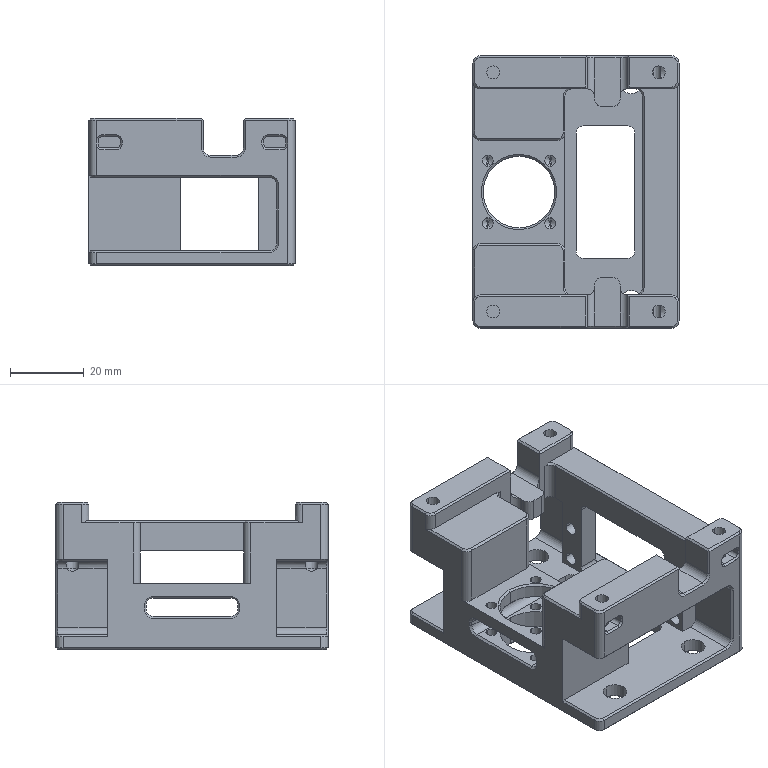NC program | Mastercam | posted with a generic post | part box 56 x 74 x 40 mm
Lines 2694 to 4682 of 45205, first 1710 of 1989 lines:
(4 FEM |TOOL - 4|DIA. OFF. - 4|LEN. - 4|TOOL DIA. - 4.)
N5436 T4 M6
N5438 G0 G54 G90 X22.359 Y9.943 C0. B0. S7000 M3
N5440 G43 H4 Z50.
N5442 Z3.054
N5444 G1 Z2.554 F600.
N5446 X22.37 Z2.345 F3000.
N5448 X22.402 Z2.138
N5450 X22.456 Z1.936
N5452 X22.531 Z1.74
N5454 X22.627 Z1.554
N5456 X22.741 Z1.378
N5458 X22.872 Z1.216
N5460 X23.02 Z1.068
N5462 X23.183 Z.936
N5464 X23.359 Z.822
N5466 X23.545 Z.727
N5468 X23.741 Z.652
N5470 X23.943 Z.598
N5472 X24.15 Z.565
N5474 X24.359 Z.554
N5476 X24.568 Y9.954 Z.517
N5478 X24.774 Y9.987 Z.48
N5480 X24.977 Y10.041 Z.443
N5482 X25.172 Y10.116 Z.406
N5484 X25.359 Y10.211 Z.369
N5486 X25.534 Y10.325 Z.332
N5488 X25.697 Y10.457 Z.295
N5490 X25.845 Y10.605 Z.259
N5492 X25.977 Y10.768 Z.222
N5494 X26.091 Y10.943 Z.185
N5496 X26.186 Y11.13 Z.148
N5498 X26.261 Y11.325 Z.111
N5500 X26.315 Y11.527 Z.074
N5502 X26.348 Y11.734 Z.037
N5504 X26.359 Y11.943 Z0.
N5506 Y13.91
N5508 X26.345 Y14.061
N5510 X26.304 Y14.175
N5512 X26.225 Y14.269
N5514 X26.061 Y14.345
N5516 X24.136 Y14.359
N5518 X24.077 Y14.358 Z-.001
N5520 X24.017 Y14.355 Z-.004
N5522 X23.958 Y14.35 Z-.01
N5524 X23.9 Y14.343 Z-.017
N5526 X23.843 Y14.335 Z-.026
N5528 X23.787 Y14.324 Z-.036
N5530 X23.732 Y14.313 Z-.048
N5532 X23.678 Y14.3 Z-.061
N5534 X23.627 Y14.286 Z-.075
N5536 X23.578 Y14.27 Z-.09
N5538 X23.531 Y14.254 Z-.106
N5540 X23.486 Y14.237 Z-.123
N5542 X23.444 Y14.22 Z-.14
N5544 X23.406 Y14.202 Z-.158
N5546 X23.37 Y14.184 Z-.176
N5548 X23.338 Y14.166 Z-.194
N5550 X23.31 Y14.147 Z-.213
N5552 X23.286 Y14.129 Z-.231
N5554 X23.265 Y14.111 Z-.248
N5556 X23.25 Y14.094 Z-.266
N5558 X23.239 Y14.077 Z-.283
N5560 X23.235 Y14.069 Z-.291
N5562 X23.233 Y14.061 Z-.299
N5564 X23.231 Y14.053 Z-.306
N5566 X23.232 Y14.045 Z-.314
N5568 X23.233 Y14.038 Z-.321
N5570 X23.236 Y14.031 Z-.328
N5572 X23.24 Y14.024 Z-.335
N5574 X23.246 Y14.018 Z-.341
N5576 X23.253 Y14.012 Z-.347
N5578 X23.262 Y14.006 Z-.353
N5580 X23.272 Y14.001 Z-.358
N5582 X23.284 Y13.995 Z-.363
N5584 X23.312 Y13.987 Z-.372
N5586 X23.347 Y13.979 Z-.379
N5588 X23.388 Y13.974 Z-.385
N5590 X23.437 Y13.971 Z-.388
N5592 X23.493 Y13.97 Z-.389
N5594 X25.91
N5596 X25.965 Y13.965
N5598 X25.97 Y13.908
N5600 Y11.623
N5602 X25.969 Y11.571 Z-.393
N5604 X25.967 Y11.569 Z-.394
N5606 Y11.568
N5608 Y11.565
N5610 Y11.559 Z-.395
N5612 X25.965 Y11.547 Z-.398
N5614 X25.96 Y11.526 Z-.402
N5616 X25.95 Y11.488 Z-.412
N5618 X25.934 Y11.456 Z-.428
N5620 X25.927 Y11.432 Z-.435
N5622 X25.921 Y11.415 Z-.443
N5624 X25.915 Y11.404 Z-.452
N5626 X25.912 Y11.402 Z-.459
N5628 X25.909 Y11.401 Z-.466
N5630 X25.905 Y11.402 Z-.477
N5632 X25.903 Y11.404 Z-.62
N5634 Y11.415 Z-.655
N5636 X25.902 Y11.432 Z-.688
N5638 Y11.456 Z-.717
N5640 Y11.488 Z-.742
N5642 X25.901 Y11.526 Z-.761
N5644 Y11.531 Z-.763
N5646 X25.903 Y11.532
N5648 X25.902 Y11.534 Z-.764
N5650 Y11.536 Z-.765
N5652 Y11.547 Z-.768
N5654 X25.901 Y11.571 Z-.773
N5656 X25.9 Y11.623 Z-.778
N5658 Y13.9
N5660 X23.493
N5662 X23.397 Z-.794
N5664 X23.328 Z-.839
N5666 X23.287 Z-.901
N5668 X23.274 Z-.972
N5670 X23.287 Z-1.044
N5672 X23.328 Z-1.106
N5674 X23.397 Z-1.15
N5676 X23.493 Z-1.167
N5678 X25.9
N5680 Y11.623
N5682 Y11.527 Z-1.183
N5684 Y11.459 Z-1.227
N5686 Y11.418 Z-1.29
N5688 Y11.404 Z-1.361
N5690 Y11.418 Z-1.433
N5692 Y11.459 Z-1.495
N5694 Y11.527 Z-1.539
N5696 Y11.623 Z-1.556
N5698 Y13.9
N5700 X23.493
N5702 X23.397 Z-1.572
N5704 X23.328 Z-1.616
N5706 X23.287 Z-1.679
N5708 X23.274 Z-1.75
N5710 X23.287 Z-1.821
N5712 X23.328 Z-1.884
N5714 X23.397 Z-1.928
N5716 X23.493 Z-1.944
N5718 X25.9
N5720 Y11.623
N5722 Y11.527 Z-1.961
N5724 Y11.459 Z-2.005
N5726 Y11.418 Z-2.067
N5728 Y11.404 Z-2.139
N5730 Y11.418 Z-2.21
N5732 Y11.459 Z-2.273
N5734 Y11.527 Z-2.317
N5736 Y11.623 Z-2.333
N5738 Y13.9
N5740 X23.493
N5742 X23.397 Z-2.35
N5744 X23.328 Z-2.394
N5746 X23.287 Z-2.456
N5748 X23.274 Z-2.528
N5750 X23.287 Z-2.599
N5752 X23.328 Z-2.661
N5754 X23.397 Z-2.706
N5756 X23.493 Z-2.722
N5758 X25.9
N5760 Y11.623
N5762 Y11.527 Z-2.739
N5764 Y11.459 Z-2.783
N5766 Y11.418 Z-2.845
N5768 Y11.404 Z-2.917
N5770 Y11.418 Z-2.988
N5772 Y11.459 Z-3.05
N5774 Y11.527 Z-3.094
N5776 Y11.623 Z-3.111
N5778 Y13.9
N5780 X23.493
N5782 X23.397 Z-3.128
N5784 X23.328 Z-3.172
N5786 X23.287 Z-3.234
N5788 X23.274 Z-3.306
N5790 X23.287 Z-3.377
N5792 X23.328 Z-3.439
N5794 X23.397 Z-3.483
N5796 X23.493 Z-3.5
N5798 X25.9
N5800 Y11.623
N5802 Y11.57 Z-3.504
N5804 Y11.525 Z-3.517
N5806 Y11.454 Z-3.563
N5808 Y11.412 Z-3.627
N5810 Y11.398 Z-3.7
N5812 Y11.412 Z-3.773
N5814 Y11.454 Z-3.837
N5816 Y11.525 Z-3.883
N5818 Y11.57 Z-3.896
N5820 Y11.623 Z-3.9
N5822 Y13.898
N5824 X25.898 Y13.9
N5826 X23.493
N5828 X23.283 Y13.889 Z-3.863
N5830 X23.077 Y13.856 Z-3.826
N5832 X22.875 Y13.802 Z-3.789
N5834 X22.679 Y13.727 Z-3.752
N5836 X22.493 Y13.632 Z-3.715
N5838 X22.317 Y13.518 Z-3.678
N5840 X22.154 Y13.386 Z-3.641
N5842 X22.006 Y13.238 Z-3.605
N5844 X21.875 Y13.076 Z-3.568
N5846 X21.76 Y12.9 Z-3.531
N5848 X21.665 Y12.713 Z-3.494
N5850 X21.59 Y12.518 Z-3.457
N5852 X21.536 Y12.316 Z-3.42
N5854 X21.503 Y12.109 Z-3.383
N5856 X21.493 Y11.9 Z-3.346
N5858 Y11.691 Z-3.335
N5860 Y11.484 Z-3.302
N5862 Y11.282 Z-3.248
N5864 Y11.087 Z-3.173
N5866 Y10.9 Z-3.078
N5868 Y10.724 Z-2.964
N5870 Y10.562 Z-2.832
N5872 Y10.414 Z-2.684
N5874 Y10.282 Z-2.522
N5876 Y10.168 Z-2.346
N5878 Y10.073 Z-2.16
N5880 Y9.998 Z-1.964
N5882 Y9.944 Z-1.762
N5884 Y9.911 Z-1.555
N5886 Y9.9 Z-1.346
N5888 Z-.846
N5890 G0 Z50.
N5892 X10.081 Y9.623
N5894 Z-1.224
N5896 G1 Z-1.724 F600.
N5898 X10.092 Z-1.933 F3000.
N5900 X10.125 Z-2.14
N5902 X10.179 Z-2.342
N5904 X10.254 Z-2.537
N5906 X10.349 Z-2.724
N5908 X10.463 Z-2.899
N5910 X10.595 Z-3.062
N5912 X10.743 Z-3.21
N5914 X10.905 Z-3.342
N5916 X11.081 Z-3.456
N5918 X11.267 Z-3.551
N5920 X11.463 Z-3.626
N5922 X11.665 Z-3.68
N5924 X11.872 Z-3.713
N5926 X12.081 Z-3.724
N5928 X12.29 Y9.634 Z-3.761
N5930 X12.497 Y9.667 Z-3.798
N5932 X12.699 Y9.721 Z-3.835
N5934 X12.894 Y9.796 Z-3.872
N5936 X13.081 Y9.891 Z-3.908
N5938 X13.256 Y10.005 Z-3.945
N5940 X13.419 Y10.137 Z-3.982
N5942 X13.567 Y10.285 Z-4.019
N5944 X13.699 Y10.447 Z-4.056
N5946 X13.813 Y10.623 Z-4.093
N5948 X13.908 Y10.81 Z-4.13
N5950 X13.983 Y11.005 Z-4.167
N5952 X14.037 Y11.207 Z-4.204
N5954 X14.07 Y11.414 Z-4.241
N5956 X14.081 Y11.623 Z-4.278
N5958 Y13.9
N5960 X11.585
N5962 X11.49 Z-4.294
N5964 X11.421 Z-4.339
N5966 X11.38 Z-4.401
N5968 X11.367 Z-4.472
N5970 X11.38 Z-4.544
N5972 X11.421 Z-4.606
N5974 X11.49 Z-4.65
N5976 X11.585 Z-4.667
N5978 X13.9
N5980 Y11.623
N5982 Y11.527 Z-4.683
N5984 Y11.459 Z-4.727
N5986 Y11.418 Z-4.79
N5988 Y11.404 Z-4.861
N5990 Y11.418 Z-4.933
N5992 Y11.459 Z-4.995
N5994 Y11.527 Z-5.039
N5996 Y11.623 Z-5.056
N5998 Y13.9
N6000 X11.585
N6002 X11.49 Z-5.072
N6004 X11.421 Z-5.116
N6006 X11.38 Z-5.179
N6008 X11.367 Z-5.25
N6010 X11.38 Z-5.321
N6012 X11.421 Z-5.384
N6014 X11.49 Z-5.428
N6016 X11.585 Z-5.444
N6018 X13.9
N6020 Y11.623
N6022 Y11.527 Z-5.461
N6024 Y11.459 Z-5.505
N6026 Y11.418 Z-5.567
N6028 Y11.404 Z-5.639
N6030 Y11.418 Z-5.71
N6032 Y11.459 Z-5.773
N6034 Y11.527 Z-5.817
N6036 Y11.623 Z-5.833
N6038 Y13.9
N6040 X11.585
N6042 X11.49 Z-5.85
N6044 X11.421 Z-5.894
N6046 X11.38 Z-5.956
N6048 X11.367 Z-6.028
N6050 X11.38 Z-6.099
N6052 X11.421 Z-6.161
N6054 X11.49 Z-6.206
N6056 X11.585 Z-6.222
N6058 X13.9
N6060 Y11.623
N6062 Y11.527 Z-6.239
N6064 Y11.459 Z-6.283
N6066 Y11.418 Z-6.345
N6068 Y11.404 Z-6.417
N6070 Y11.418 Z-6.488
N6072 Y11.459 Z-6.55
N6074 Y11.527 Z-6.594
N6076 Y11.623 Z-6.611
N6078 Y13.9
N6080 X11.585
N6082 X11.49 Z-6.628
N6084 X11.421 Z-6.672
N6086 X11.38 Z-6.734
N6088 X11.367 Z-6.806
N6090 X11.38 Z-6.877
N6092 X11.421 Z-6.939
N6094 X11.49 Z-6.983
N6096 X11.585 Z-7.
N6098 X13.9
N6100 Y11.623
N6102 Y11.527 Z-7.017
N6104 Y11.459 Z-7.061
N6106 Y11.418 Z-7.123
N6108 Y11.404 Z-7.194
N6110 Y11.418 Z-7.266
N6112 Y11.459 Z-7.328
N6114 Y11.527 Z-7.372
N6116 Y11.623 Z-7.389
N6118 Y13.9
N6120 X11.585
N6122 X11.49 Z-7.406
N6124 X11.421 Z-7.45
N6126 X11.38 Z-7.512
N6128 X11.367 Z-7.583
N6130 X11.38 Z-7.655
N6132 X11.421 Z-7.717
N6134 X11.49 Z-7.761
N6136 X11.585 Z-7.778
N6138 X13.9
N6140 Y11.623
N6142 Y11.527 Z-7.794
N6144 Y11.459 Z-7.839
N6146 Y11.418 Z-7.901
N6148 Y11.404 Z-7.972
N6150 Y11.418 Z-8.044
N6152 Y11.459 Z-8.106
N6154 Y11.527 Z-8.15
N6156 Y11.623 Z-8.167
N6158 Y13.9
N6160 X11.585
N6162 X11.49 Z-8.183
N6164 X11.421 Z-8.227
N6166 X11.38 Z-8.29
N6168 X11.367 Z-8.361
N6170 X11.38 Z-8.433
N6172 X11.421 Z-8.495
N6174 X11.49 Z-8.539
N6176 X11.585 Z-8.556
N6178 X13.9
N6180 Y11.623
N6182 Y11.527 Z-8.572
N6184 Y11.459 Z-8.616
N6186 Y11.418 Z-8.679
N6188 Y11.404 Z-8.75
N6190 Y11.418 Z-8.821
N6192 Y11.459 Z-8.884
N6194 Y11.527 Z-8.928
N6196 Y11.623 Z-8.944
N6198 Y13.9
N6200 X11.585
N6202 X11.49 Z-8.961
N6204 X11.421 Z-9.005
N6206 X11.38 Z-9.067
N6208 X11.367 Z-9.139
N6210 X11.38 Z-9.21
N6212 X11.421 Z-9.273
N6214 X11.49 Z-9.317
N6216 X11.585 Z-9.333
N6218 X13.9
N6220 Y11.623
N6222 Y11.527 Z-9.35
N6224 Y11.459 Z-9.394
N6226 Y11.418 Z-9.456
N6228 Y11.404 Z-9.528
N6230 Y11.418 Z-9.599
N6232 Y11.459 Z-9.661
N6234 Y11.527 Z-9.706
N6236 Y11.623 Z-9.722
N6238 Y13.9
N6240 X11.585
N6242 X11.49 Z-9.739
N6244 X11.421 Z-9.783
N6246 X11.38 Z-9.845
N6248 X11.367 Z-9.917
N6250 X11.38 Z-9.988
N6252 X11.421 Z-10.05
N6254 X11.489 Z-10.094
N6256 X11.585 Z-10.111
N6258 X13.9 Y13.897
N6260 Y11.623
N6262 Y11.527 Z-10.128
N6264 Y11.459 Z-10.172
N6266 Y11.418 Z-10.234
N6268 Y11.404 Z-10.306
N6270 Y11.418 Z-10.377
N6272 Y11.459 Z-10.439
N6274 Y11.527 Z-10.483
N6276 Y11.623 Z-10.5
N6278 Y13.897
N6280 X11.585 Y13.9
N6282 X11.376 Y13.889 Z-10.463
N6284 X11.169 Y13.857 Z-10.426
N6286 X10.967 Y13.803 Z-10.389
N6288 X10.771 Y13.728 Z-10.352
N6290 X10.585 Y13.633 Z-10.315
N6292 X10.409 Y13.52 Z-10.278
N6294 X10.246 Y13.388 Z-10.241
N6296 X10.098 Y13.24 Z-10.205
N6298 X9.966 Y13.078 Z-10.168
N6300 X9.852 Y12.902 Z-10.131
N6302 X9.756 Y12.716 Z-10.094
N6304 X9.681 Y12.521 Z-10.057
N6306 X9.627 Y12.319 Z-10.02
N6308 X9.594 Y12.112 Z-9.983
N6310 X9.582 Y11.903 Z-9.946
N6312 Y11.694 Z-9.935
N6314 Y11.487 Z-9.902
N6316 Y11.285 Z-9.848
N6318 X9.581 Y11.089 Z-9.773
N6320 Y10.903 Z-9.678
N6322 Y10.727 Z-9.564
N6324 Y10.564 Z-9.432
N6326 X9.58 Y10.416 Z-9.284
N6328 Y10.285 Z-9.122
N6330 Y10.171 Z-8.946
N6332 Y10.076 Z-8.76
N6334 Y10.001 Z-8.564
N6336 Y9.946 Z-8.362
N6338 Y9.914 Z-8.155
N6340 Y9.903 Z-7.946
N6342 Z-7.446
N6344 G0 Z50.
N6346 X10.081 Y-.543
N6348 Z-1.224
N6350 G1 Z-1.724 F600.
N6352 X10.092 Z-1.933 F3000.
N6354 X10.125 Z-2.14
N6356 X10.179 Z-2.342
N6358 X10.254 Z-2.537
N6360 X10.349 Z-2.724
N6362 X10.463 Z-2.899
N6364 X10.595 Z-3.062
N6366 X10.743 Z-3.21
N6368 X10.905 Z-3.342
N6370 X11.081 Z-3.456
N6372 X11.267 Z-3.551
N6374 X11.463 Z-3.626
N6376 X11.665 Z-3.68
N6378 X11.872 Z-3.713
N6380 X12.081 Z-3.724
N6382 X12.29 Y-.554 Z-3.761
N6384 X12.497 Y-.587 Z-3.798
N6386 X12.699 Y-.641 Z-3.835
N6388 X12.894 Y-.716 Z-3.872
N6390 X13.081 Y-.811 Z-3.908
N6392 X13.256 Y-.925 Z-3.945
N6394 X13.419 Y-1.057 Z-3.982
N6396 X13.567 Y-1.205 Z-4.019
N6398 X13.699 Y-1.367 Z-4.056
N6400 X13.813 Y-1.543 Z-4.093
N6402 X13.908 Y-1.729 Z-4.13
N6404 X13.983 Y-1.925 Z-4.167
N6406 X14.037 Y-2.127 Z-4.204
N6408 X14.07 Y-2.334 Z-4.241
N6410 X14.081 Y-2.543 Z-4.278
N6412 Y-4.9
N6414 X11.666
N6416 X11.57 Z-4.294
N6418 X11.502 Z-4.339
N6420 X11.461 Z-4.401
N6422 X11.447 Z-4.472
N6424 X11.461 Z-4.544
N6426 X11.502 Z-4.606
N6428 X11.57 Z-4.65
N6430 X11.666 Z-4.667
N6432 X13.9
N6434 Y-2.543
N6436 Y-2.447 Z-4.683
N6438 Y-2.379 Z-4.727
N6440 Y-2.338 Z-4.79
N6442 Y-2.324 Z-4.861
N6444 Y-2.338 Z-4.933
N6446 Y-2.379 Z-4.995
N6448 Y-2.447 Z-5.039
N6450 Y-2.543 Z-5.056
N6452 Y-4.9
N6454 X11.666
N6456 X11.57 Z-5.072
N6458 X11.502 Z-5.116
N6460 X11.461 Z-5.179
N6462 X11.447 Z-5.25
N6464 X11.461 Z-5.321
N6466 X11.502 Z-5.384
N6468 X11.57 Z-5.428
N6470 X11.666 Z-5.444
N6472 X13.9
N6474 Y-2.543
N6476 Y-2.447 Z-5.461
N6478 Y-2.379 Z-5.505
N6480 Y-2.338 Z-5.567
N6482 Y-2.324 Z-5.639
N6484 Y-2.338 Z-5.71
N6486 Y-2.379 Z-5.773
N6488 Y-2.447 Z-5.817
N6490 Y-2.543 Z-5.833
N6492 Y-4.9
N6494 X11.666
N6496 X11.57 Z-5.85
N6498 X11.502 Z-5.894
N6500 X11.461 Z-5.956
N6502 X11.447 Z-6.028
N6504 X11.461 Z-6.099
N6506 X11.502 Z-6.161
N6508 X11.57 Z-6.206
N6510 X11.666 Z-6.222
N6512 X13.9
N6514 Y-2.543
N6516 Y-2.447 Z-6.239
N6518 Y-2.379 Z-6.283
N6520 Y-2.338 Z-6.345
N6522 Y-2.324 Z-6.417
N6524 Y-2.338 Z-6.488
N6526 Y-2.379 Z-6.55
N6528 Y-2.447 Z-6.594
N6530 Y-2.543 Z-6.611
N6532 Y-4.9
N6534 X11.666
N6536 X11.57 Z-6.628
N6538 X11.502 Z-6.672
N6540 X11.461 Z-6.734
N6542 X11.447 Z-6.806
N6544 X11.461 Z-6.877
N6546 X11.502 Z-6.939
N6548 X11.57 Z-6.983
N6550 X11.666 Z-7.
N6552 X13.9
N6554 Y-2.543
N6556 Y-2.447 Z-7.017
N6558 Y-2.379 Z-7.061
N6560 Y-2.338 Z-7.123
N6562 Y-2.324 Z-7.194
N6564 Y-2.338 Z-7.266
N6566 Y-2.379 Z-7.328
N6568 Y-2.447 Z-7.372
N6570 Y-2.543 Z-7.389
N6572 Y-4.9
N6574 X11.666
N6576 X11.57 Z-7.406
N6578 X11.502 Z-7.45
N6580 X11.461 Z-7.512
N6582 X11.447 Z-7.583
N6584 X11.461 Z-7.655
N6586 X11.502 Z-7.717
N6588 X11.57 Z-7.761
N6590 X11.666 Z-7.778
N6592 X13.9
N6594 Y-2.543
N6596 Y-2.447 Z-7.794
N6598 Y-2.379 Z-7.839
N6600 Y-2.338 Z-7.901
N6602 Y-2.324 Z-7.972
N6604 Y-2.338 Z-8.044
N6606 Y-2.379 Z-8.106
N6608 Y-2.447 Z-8.15
N6610 Y-2.543 Z-8.167
N6612 Y-4.9
N6614 X11.666
N6616 X11.57 Z-8.183
N6618 X11.502 Z-8.227
N6620 X11.461 Z-8.29
N6622 X11.447 Z-8.361
N6624 X11.461 Z-8.433
N6626 X11.502 Z-8.495
N6628 X11.57 Z-8.539
N6630 X11.666 Z-8.556
N6632 X13.9
N6634 Y-2.543
N6636 Y-2.447 Z-8.572
N6638 Y-2.379 Z-8.616
N6640 Y-2.338 Z-8.679
N6642 Y-2.324 Z-8.75
N6644 Y-2.338 Z-8.821
N6646 Y-2.379 Z-8.884
N6648 Y-2.447 Z-8.928
N6650 Y-2.543 Z-8.944
N6652 Y-4.9
N6654 X11.666
N6656 X11.57 Z-8.961
N6658 X11.502 Z-9.005
N6660 X11.461 Z-9.067
N6662 X11.447 Z-9.139
N6664 X11.461 Z-9.21
N6666 X11.502 Z-9.273
N6668 X11.57 Z-9.317
N6670 X11.666 Z-9.333
N6672 X13.9
N6674 Y-2.543
N6676 Y-2.447 Z-9.35
N6678 Y-2.379 Z-9.394
N6680 Y-2.338 Z-9.456
N6682 Y-2.324 Z-9.528
N6684 Y-2.338 Z-9.599
N6686 Y-2.379 Z-9.661
N6688 Y-2.447 Z-9.706
N6690 Y-2.543 Z-9.722
N6692 Y-4.9
N6694 X11.666
N6696 X11.57 Z-9.739
N6698 X11.502 Z-9.783
N6700 X11.461 Z-9.845
N6702 X11.447 Z-9.917
N6704 X11.461 Z-9.988
N6706 X11.502 Z-10.05
N6708 X11.57 Z-10.094
N6710 X11.666 Z-10.111
N6712 X13.897
N6714 X13.9 Y-2.543
N6716 Y-2.447 Z-10.128
N6718 Y-2.379 Z-10.172
N6720 Y-2.338 Z-10.234
N6722 Y-2.324 Z-10.306
N6724 Y-2.338 Z-10.377
N6726 Y-2.379 Z-10.439
N6728 Y-2.447 Z-10.483
N6730 Y-2.543 Z-10.5
N6732 X13.897 Y-4.9
N6734 X11.666
N6736 X11.353 Y-4.875 Z-10.445
N6738 X11.048 Y-4.802 Z-10.389
N6740 X10.758 Y-4.682 Z-10.334
N6742 X10.49 Y-4.518 Z-10.278
N6744 X10.252 Y-4.314 Z-10.223
N6746 X10.048 Y-4.076 Z-10.168
N6748 X9.884 Y-3.808 Z-10.112
N6750 X9.764 Y-3.518 Z-10.057
N6752 X9.69 Y-3.213 Z-10.001
N6754 X9.666 Y-2.9 Z-9.946
N6756 Y-2.691 Z-9.935
N6758 Y-2.484 Z-9.902
N6760 Y-2.282 Z-9.848
N6762 Y-2.087 Z-9.773
N6764 Y-1.9 Z-9.678
N6766 Y-1.724 Z-9.564
N6768 Y-1.562 Z-9.432
N6770 Y-1.414 Z-9.284
N6772 Y-1.282 Z-9.122
N6774 Y-1.168 Z-8.946
N6776 Y-1.073 Z-8.76
N6778 Y-.998 Z-8.564
N6780 Y-.944 Z-8.362
N6782 Y-.911 Z-8.155
N6784 Y-.9 Z-7.946
N6786 Z-7.446
N6788 G0 Z50.
N6790 X22.217 Y-1.359
N6792 Z3.054
N6794 G1 Z2.554 F600.
N6796 Y-1.37 Z2.345 F3000.
N6798 Y-1.402 Z2.138
N6800 Y-1.456 Z1.936
N6802 Y-1.531 Z1.74
N6804 Y-1.627 Z1.554
N6806 Y-1.741 Z1.378
N6808 Y-1.872 Z1.216
N6810 Y-2.02 Z1.068
N6812 Y-2.183 Z.936
N6814 Y-2.359 Z.822
N6816 Y-2.545 Z.727
N6818 Y-2.741 Z.652
N6820 Y-2.943 Z.598
N6822 Y-3.15 Z.565
N6824 Y-3.359 Z.554
N6826 X22.228 Y-3.568 Z.517
N6828 X22.26 Y-3.774 Z.48
N6830 X22.315 Y-3.977 Z.443
N6832 X22.39 Y-4.172 Z.406
N6834 X22.485 Y-4.359 Z.369
N6836 X22.599 Y-4.534 Z.332
N6838 X22.73 Y-4.697 Z.295
N6840 X22.878 Y-4.845 Z.259
N6842 X23.041 Y-4.977 Z.222
N6844 X23.217 Y-5.091 Z.185
N6846 X23.403 Y-5.186 Z.148
N6848 X23.599 Y-5.261 Z.111
N6850 X23.801 Y-5.315 Z.074
N6852 X24.008 Y-5.348 Z.037
N6854 X24.217 Y-5.359 Z0.
N6856 X25.91
N6858 X26.061 Y-5.345
N6860 X26.175 Y-5.304
N6862 X26.304 Y-5.175
N6864 X26.345 Y-5.061
N6866 X26.359 Y-2.863
N6868 X26.358 Y-2.819 Z-.001
N6870 X26.355 Y-2.776 Z-.004
N6872 X26.35 Y-2.734 Z-.01
N6874 X26.343 Y-2.693 Z-.017
N6876 X26.334 Y-2.653 Z-.026
N6878 X26.324 Y-2.615 Z-.036
N6880 X26.312 Y-2.579 Z-.048
N6882 X26.299 Y-2.545 Z-.061
N6884 X26.285 Y-2.512 Z-.075
N6886 X26.27 Y-2.481 Z-.09
N6888 X26.254 Y-2.453 Z-.106
N6890 X26.237 Y-2.426 Z-.123
N6892 X26.219 Y-2.402 Z-.14
N6894 X26.202 Y-2.381 Z-.158
N6896 X26.183 Y-2.361 Z-.176
N6898 X26.165 Y-2.345 Z-.194
N6900 X26.147 Y-2.331 Z-.213
N6902 X26.129 Y-2.321 Z-.231
N6904 X26.111 Y-2.313 Z-.248
N6906 X26.093 Y-2.309 Z-.266
N6908 X26.077 Y-2.307 Z-.283
N6910 X26.06 Y-2.31 Z-.299
N6912 X26.045 Y-2.315 Z-.314
N6914 X26.031 Y-2.325 Z-.328
N6916 X26.018 Y-2.338 Z-.341
N6918 X26.006 Y-2.354 Z-.353
N6920 X25.995 Y-2.375 Z-.363
N6922 X25.987 Y-2.4 Z-.372
N6924 X25.979 Y-2.429 Z-.379
N6926 X25.974 Y-2.463 Z-.385
N6928 X25.971 Y-2.501 Z-.388
N6930 X25.97 Y-2.543 Z-.389
N6932 Y-4.908
N6934 X25.965 Y-4.965
N6936 X25.91 Y-4.97
N6938 X23.573
N6940 X23.521 Y-4.969 Z-.393
N6942 X23.519 Y-4.967 Z-.394
N6944 X23.518
N6946 X23.515
N6948 X23.509 Z-.395
N6950 X23.497 Y-4.965 Z-.398
N6952 X23.476 Y-4.96 Z-.402
N6954 X23.438 Y-4.95 Z-.412
N6956 X23.406 Y-4.934 Z-.428
N6958 X23.382 Y-4.927 Z-.435
N6960 X23.365 Y-4.921 Z-.443
N6962 X23.354 Y-4.915 Z-.452
N6964 X23.352 Y-4.912 Z-.459
N6966 X23.351 Y-4.909 Z-.466
N6968 X23.352 Y-4.905 Z-.477
N6970 X23.354 Y-4.903 Z-.62
N6972 X23.365 Z-.655
N6974 X23.382 Y-4.902 Z-.688
N6976 X23.406 Z-.717
N6978 X23.438 Z-.742
N6980 X23.476 Y-4.901 Z-.761
N6982 X23.481 Z-.763
N6984 X23.482 Y-4.903
N6986 X23.484 Y-4.902 Z-.764
N6988 X23.486 Z-.765
N6990 X23.497 Z-.768
N6992 X23.521 Y-4.901 Z-.773
N6994 X23.573 Y-4.9 Z-.778
N6996 X25.9
N6998 Y-2.543
N7000 Y-2.447 Z-.794
N7002 Y-2.379 Z-.839
N7004 Y-2.338 Z-.901
N7006 Y-2.324 Z-.972
N7008 Y-2.338 Z-1.044
N7010 Y-2.379 Z-1.106
N7012 Y-2.447 Z-1.15
N7014 Y-2.543 Z-1.167
N7016 Y-4.9
N7018 X23.573
N7020 X23.477 Z-1.183
N7022 X23.409 Z-1.227
N7024 X23.368 Z-1.29
N7026 X23.354 Z-1.361
N7028 X23.368 Z-1.433
N7030 X23.409 Z-1.495
N7032 X23.477 Z-1.539
N7034 X23.573 Z-1.556
N7036 X25.9
N7038 Y-2.543
N7040 Y-2.447 Z-1.572
N7042 Y-2.379 Z-1.616
N7044 Y-2.338 Z-1.679
N7046 Y-2.324 Z-1.75
N7048 Y-2.338 Z-1.821
N7050 Y-2.379 Z-1.884
N7052 Y-2.447 Z-1.928
N7054 Y-2.543 Z-1.944
N7056 Y-4.9
N7058 X23.573
N7060 X23.477 Z-1.961
N7062 X23.409 Z-2.005
N7064 X23.368 Z-2.067
N7066 X23.354 Z-2.139
N7068 X23.368 Z-2.21
N7070 X23.409 Z-2.273
N7072 X23.477 Z-2.317
N7074 X23.573 Z-2.333
N7076 X25.9
N7078 Y-2.543
N7080 Y-2.447 Z-2.35
N7082 Y-2.379 Z-2.394
N7084 Y-2.338 Z-2.456
N7086 Y-2.324 Z-2.528
N7088 Y-2.338 Z-2.599
N7090 Y-2.379 Z-2.661
N7092 Y-2.447 Z-2.706
N7094 Y-2.543 Z-2.722
N7096 Y-4.9
N7098 X23.573
N7100 X23.477 Z-2.739
N7102 X23.409 Z-2.783
N7104 X23.368 Z-2.845
N7106 X23.354 Z-2.917
N7108 X23.368 Z-2.988
N7110 X23.409 Z-3.05
N7112 X23.477 Z-3.094
N7114 X23.573 Z-3.111
N7116 X25.9
N7118 Y-2.543
N7120 Y-2.447 Z-3.128
N7122 Y-2.379 Z-3.172
N7124 Y-2.338 Z-3.234
N7126 Y-2.324 Z-3.306
N7128 Y-2.338 Z-3.377
N7130 Y-2.379 Z-3.439
N7132 Y-2.447 Z-3.483
N7134 Y-2.543 Z-3.5
N7136 Y-4.9
N7138 X23.573
N7140 X23.52 Z-3.504
N7142 X23.475 Z-3.517
N7144 X23.404 Z-3.563
N7146 X23.362 Z-3.627
N7148 X23.348 Z-3.7
N7150 X23.362 Z-3.773
N7152 X23.404 Z-3.837
N7154 X23.475 Z-3.883
N7156 X23.52 Z-3.896
N7158 X23.573 Z-3.9
N7160 X25.898
N7162 X25.9 Y-2.543
N7164 X25.889 Y-2.334 Z-3.863
N7166 X25.857 Y-2.127 Z-3.826
N7168 X25.803 Y-1.925 Z-3.789
N7170 X25.728 Y-1.729 Z-3.752
N7172 X25.633 Y-1.543 Z-3.715
N7174 X25.519 Y-1.367 Z-3.678
N7176 X25.387 Y-1.204 Z-3.641
N7178 X25.24 Y-1.056 Z-3.605
N7180 X25.077 Y-.924 Z-3.568
N7182 X24.901 Y-.81 Z-3.531
N7184 X24.715 Y-.715 Z-3.494
N7186 X24.52 Y-.64 Z-3.457
N7188 X24.318 Y-.585 Z-3.42
N7190 X24.111 Y-.552 Z-3.383
N7192 X23.902 Y-.541 Z-3.346
N7194 X23.693 Z-3.335
N7196 X23.486 Z-3.302
N7198 X23.284 Z-3.248
N7200 X23.088 Z-3.173
N7202 X22.902 Y-.54 Z-3.078
N7204 X22.726 Z-2.964
N7206 X22.563 Z-2.832
N7208 X22.415 Z-2.684
N7210 X22.284 Z-2.522
N7212 X22.17 Z-2.346
N7214 X22.075 Z-2.16
N7216 X22. Z-1.964
N7218 X21.945 Z-1.762
N7220 X21.913 Z-1.555
N7222 X21.902 Z-1.346
N7224 Z-.846
N7226 G0 Z50.
N7228 X-9.585 Y-.9
N7230 Z-1.224
N7232 G1 Z-1.724 F600.
N7234 Y-.911 Z-1.933 F3000.
N7236 Y-.944 Z-2.14
N7238 Y-.998 Z-2.342
N7240 Y-1.073 Z-2.537
N7242 Y-1.168 Z-2.724
N7244 Y-1.282 Z-2.899
N7246 Y-1.414 Z-3.062
N7248 Y-1.562 Z-3.21
N7250 Y-1.724 Z-3.342
N7252 Y-1.9 Z-3.456
N7254 Y-2.087 Z-3.551
N7256 Y-2.282 Z-3.626
N7258 Y-2.484 Z-3.68
N7260 Y-2.691 Z-3.713
N7262 Y-2.9 Z-3.724
N7264 X-9.596 Y-3.109 Z-3.761
N7266 X-9.629 Y-3.316 Z-3.798
N7268 X-9.683 Y-3.518 Z-3.835
N7270 X-9.758 Y-3.713 Z-3.872
N7272 X-9.853 Y-3.9 Z-3.908
N7274 X-9.967 Y-4.076 Z-3.945
N7276 X-10.099 Y-4.238 Z-3.982
N7278 X-10.247 Y-4.386 Z-4.019
N7280 X-10.41 Y-4.518 Z-4.056
N7282 X-10.585 Y-4.632 Z-4.093
N7284 X-10.772 Y-4.727 Z-4.13
N7286 X-10.967 Y-4.802 Z-4.167
N7288 X-11.17 Y-4.856 Z-4.204
N7290 X-11.376 Y-4.889 Z-4.241
N7292 X-11.585 Y-4.9 Z-4.278
N7294 X-14.081
N7296 Y-2.623
N7298 X-14.08 Y-2.594 Z-4.279
N7300 X-14.079 Y-2.566 Z-4.282
N7302 X-14.078 Y-2.554 Z-4.285
N7304 X-14.076 Y-2.552
N7306 Y-2.55
N7308 X-14.075 Y-2.547 Z-4.286
N7310 Y-2.541 Z-4.287
N7312 X-14.07 Y-2.517 Z-4.293
N7314 X-14.062 Y-2.496 Z-4.3
N7316 X-14.056 Y-2.476 Z-4.306
N7318 X-14.047 Y-2.458 Z-4.315
N7320 X-14.038 Y-2.442 Z-4.325
N7322 X-14.026 Y-2.428 Z-4.336
N7324 X-14.016 Y-2.416 Z-4.346
N7326 X-14.005 Y-2.405 Z-4.357
N7328 X-13.997 Y-2.397 Z-4.365
N7330 X-13.989 Y-2.39 Z-4.373
N7332 X-13.981 Y-2.386 Z-4.381
N7334 X-13.973 Y-2.383 Z-4.39
N7336 X-13.964 Y-2.382 Z-4.398
N7338 X-13.956 Y-2.383 Z-4.407
N7340 X-13.947 Y-2.386 Z-4.415
N7342 X-13.939 Y-2.39 Z-4.423
N7344 X-13.931 Y-2.397 Z-4.431
N7346 X-13.923 Y-2.405 Z-4.44
N7348 X-13.916 Y-2.416 Z-4.451
N7350 X-13.909 Y-2.428 Z-4.466
N7352 X-13.903 Y-2.442 Z-4.606
N7354 Y-2.458 Z-4.619
N7356 Y-2.476 Z-4.631
N7358 Y-2.496 Z-4.641
N7360 Y-2.517 Z-4.65
N7362 Y-2.541 Z-4.657
N7364 Y-2.554 Z-4.66
N7366 Y-2.557 Z-4.661
N7368 Y-2.558
N7370 Y-2.56
N7372 X-13.902 Y-2.566 Z-4.662
N7374 X-13.901 Y-2.594 Z-4.666
N7376 X-13.9 Y-2.623 Z-4.667
N7378 Y-4.9
N7380 X-11.585
N7382 X-11.49 Z-4.683
N7384 X-11.421 Z-4.727
N7386 X-11.38 Z-4.79
N7388 X-11.367 Z-4.861
N7390 X-11.38 Z-4.933
N7392 X-11.421 Z-4.995
N7394 X-11.49 Z-5.039
N7396 X-11.585 Z-5.056
N7398 X-13.9
N7400 Y-2.623
N7402 Y-2.527 Z-5.072
N7404 Y-2.459 Z-5.116
N7406 Y-2.418 Z-5.179
N7408 Y-2.404 Z-5.25
N7410 Y-2.418 Z-5.321
N7412 Y-2.459 Z-5.384
N7414 Y-2.527 Z-5.428
N7416 Y-2.623 Z-5.444
N7418 Y-4.9
N7420 X-11.585
N7422 X-11.49 Z-5.461
N7424 X-11.421 Z-5.505
N7426 X-11.38 Z-5.567
N7428 X-11.367 Z-5.639
N7430 X-11.38 Z-5.71
N7432 X-11.421 Z-5.773
N7434 X-11.49 Z-5.817
N7436 X-11.585 Z-5.833
N7438 X-13.9
N7440 Y-2.623
N7442 Y-2.527 Z-5.85
N7444 Y-2.459 Z-5.894
N7446 Y-2.418 Z-5.956
N7448 Y-2.404 Z-6.028
N7450 Y-2.418 Z-6.099
N7452 Y-2.459 Z-6.161
N7454 Y-2.527 Z-6.206
N7456 Y-2.623 Z-6.222
N7458 Y-4.9
N7460 X-11.585
N7462 X-11.49 Z-6.239
N7464 X-11.421 Z-6.283
N7466 X-11.38 Z-6.345
N7468 X-11.367 Z-6.417
N7470 X-11.38 Z-6.488
N7472 X-11.421 Z-6.55
N7474 X-11.49 Z-6.594
N7476 X-11.585 Z-6.611
N7478 X-13.9
N7480 Y-2.623
N7482 Y-2.527 Z-6.628
N7484 Y-2.459 Z-6.672
N7486 Y-2.418 Z-6.734
N7488 Y-2.404 Z-6.806
N7490 Y-2.418 Z-6.877
N7492 Y-2.459 Z-6.939
N7494 Y-2.527 Z-6.983
N7496 Y-2.623 Z-7.
N7498 Y-4.9
N7500 X-11.585
N7502 X-11.49 Z-7.017
N7504 X-11.421 Z-7.061
N7506 X-11.38 Z-7.123
N7508 X-11.367 Z-7.194
N7510 X-11.38 Z-7.266
N7512 X-11.421 Z-7.328
N7514 X-11.49 Z-7.372
N7516 X-11.585 Z-7.389
N7518 X-13.9
N7520 Y-2.623
N7522 Y-2.527 Z-7.406
N7524 Y-2.459 Z-7.45
N7526 Y-2.418 Z-7.512
N7528 Y-2.404 Z-7.583
N7530 Y-2.418 Z-7.655
N7532 Y-2.459 Z-7.717
N7534 Y-2.527 Z-7.761
N7536 Y-2.623 Z-7.778
N7538 Y-4.9
N7540 X-11.585
N7542 X-11.49 Z-7.794
N7544 X-11.421 Z-7.839
N7546 X-11.38 Z-7.901
N7548 X-11.367 Z-7.972
N7550 X-11.38 Z-8.044
N7552 X-11.421 Z-8.106
N7554 X-11.49 Z-8.15
N7556 X-11.585 Z-8.167
N7558 X-13.9
N7560 Y-2.623
N7562 Y-2.527 Z-8.183
N7564 Y-2.459 Z-8.227
N7566 Y-2.418 Z-8.29
N7568 Y-2.404 Z-8.361
N7570 Y-2.418 Z-8.433
N7572 Y-2.459 Z-8.495
N7574 Y-2.527 Z-8.539
N7576 Y-2.623 Z-8.556
N7578 Y-4.9
N7580 X-11.585
N7582 X-11.49 Z-8.572
N7584 X-11.421 Z-8.616
N7586 X-11.38 Z-8.679
N7588 X-11.367 Z-8.75
N7590 X-11.38 Z-8.821
N7592 X-11.421 Z-8.884
N7594 X-11.49 Z-8.928
N7596 X-11.585 Z-8.944
N7598 X-13.9
N7600 Y-2.623
N7602 Y-2.527 Z-8.961
N7604 Y-2.459 Z-9.005
N7606 Y-2.418 Z-9.067
N7608 Y-2.404 Z-9.139
N7610 Y-2.418 Z-9.21
N7612 Y-2.459 Z-9.273
N7614 Y-2.527 Z-9.317
N7616 Y-2.623 Z-9.333
N7618 Y-4.9
N7620 X-11.585
N7622 X-11.49 Z-9.35
N7624 X-11.421 Z-9.394
N7626 X-11.38 Z-9.456
N7628 X-11.367 Z-9.528
N7630 X-11.38 Z-9.599
N7632 X-11.421 Z-9.661
N7634 X-11.49 Z-9.706
N7636 X-11.585 Z-9.722
N7638 X-13.9
N7640 Y-2.623
N7642 Y-2.527 Z-9.739
N7644 Y-2.459 Z-9.783
N7646 Y-2.418 Z-9.845
N7648 Y-2.404 Z-9.917
N7650 Y-2.418 Z-9.988
N7652 Y-2.459 Z-10.05
N7654 Y-2.527 Z-10.094
N7656 Y-2.623 Z-10.111
N7658 Y-4.897
N7660 X-11.585 Y-4.9
N7662 X-11.489 Z-10.128
N7664 X-11.421 Z-10.172
N7666 X-11.38 Z-10.234
N7668 X-11.366 Z-10.306
N7670 X-11.38 Z-10.377
N7672 X-11.421 Z-10.439
N7674 X-11.489 Z-10.483
N7676 X-11.585 Z-10.5
N7678 X-13.9 Y-4.897
N7680 Y-2.623
N7682 X-13.875 Y-2.31 Z-10.445
N7684 X-13.802 Y-2.005 Z-10.389
N7686 X-13.682 Y-1.715 Z-10.334
N7688 X-13.518 Y-1.447 Z-10.278
N7690 X-13.314 Y-1.209 Z-10.223
N7692 X-13.076 Y-1.005 Z-10.168
N7694 X-12.808 Y-.841 Z-10.112
N7696 X-12.518 Y-.721 Z-10.057
N7698 X-12.213 Y-.648 Z-10.001
N7700 X-11.9 Y-.623 Z-9.946
N7702 X-11.691 Z-9.935
N7704 X-11.484 Z-9.902
N7706 X-11.282 Z-9.848
N7708 X-11.087 Z-9.773
N7710 X-10.9 Z-9.678
N7712 X-10.724 Z-9.564
N7714 X-10.562 Z-9.432
N7716 X-10.414 Z-9.284
N7718 X-10.282 Z-9.122
N7720 X-10.168 Z-8.946
N7722 X-10.073 Z-8.76
N7724 X-9.998 Z-8.564
N7726 X-9.944 Z-8.362
N7728 X-9.911 Z-8.155
N7730 X-9.9 Z-7.946
N7732 Z-7.446
N7734 G0 Z50.
N7736 X-22.109 Y-1.372
N7738 Z3.054
N7740 G1 Z2.554 F600.
N7742 Y-1.383 Z2.345 F3000.
N7744 Y-1.416 Z2.138
N7746 Y-1.47 Z1.936
N7748 X-22.11 Y-1.545 Z1.74
N7750 X-22.111 Y-1.64 Z1.554
N7752 Y-1.754 Z1.378
N7754 X-22.112 Y-1.886 Z1.216
N7756 X-22.113 Y-2.034 Z1.068
N7758 X-22.114 Y-2.197 Z.936
N7760 X-22.116 Y-2.372 Z.822
N7762 X-22.117 Y-2.559 Z.727
N7764 X-22.118 Y-2.754 Z.652
N7766 X-22.12 Y-2.957 Z.598
N7768 X-22.121 Y-3.163 Z.565
N7770 X-22.122 Y-3.372 Z.554
N7772 X-22.135 Y-3.581 Z.517
N7774 X-22.169 Y-3.788 Z.48
N7776 X-22.225 Y-3.99 Z.443
N7778 X-22.301 Y-4.185 Z.406
N7780 X-22.397 Y-4.371 Z.369
N7782 X-22.513 Y-4.545 Z.332
N7784 X-22.645 Y-4.707 Z.295
N7786 X-22.794 Y-4.854 Z.259
N7788 X-22.958 Y-4.985 Z.222
N7790 X-23.134 Y-5.098 Z.185
N7792 X-23.322 Y-5.191 Z.148
N7794 X-23.517 Y-5.265 Z.111
N7796 X-23.72 Y-5.318 Z.074
N7798 X-23.927 Y-5.349 Z.037
N7800 X-24.136 Y-5.359 Z0.
N7802 X-26.061 Y-5.345
N7804 X-26.225 Y-5.269
N7806 X-26.304 Y-5.175
N7808 X-26.345 Y-5.061
N7810 X-26.359 Y-4.91
N7812 Y-2.943
N7814 X-26.357 Y-2.899 Z-.001
N7816 X-26.354 Y-2.856 Z-.004
N7818 X-26.349 Y-2.814 Z-.01
N7820 X-26.342 Y-2.773 Z-.017
N7822 X-26.333 Y-2.733 Z-.026
N7824 X-26.323 Y-2.695 Z-.036
N7826 X-26.311 Y-2.659 Z-.048
N7828 X-26.298 Y-2.625 Z-.061
N7830 X-26.284 Y-2.592 Z-.075
N7832 X-26.268 Y-2.561 Z-.09
N7834 X-26.252 Y-2.533 Z-.106
N7836 X-26.236 Y-2.506 Z-.123
N7838 X-26.218 Y-2.482 Z-.14
N7840 X-26.2 Y-2.461 Z-.158
N7842 X-26.182 Y-2.441 Z-.176
N7844 X-26.164 Y-2.425 Z-.194
N7846 X-26.146 Y-2.412 Z-.213
N7848 X-26.128 Y-2.401 Z-.231
N7850 X-26.11 Y-2.393 Z-.248
N7852 X-26.093 Y-2.389 Z-.266
N7854 X-26.076 Y-2.387 Z-.283
N7856 X-26.06 Y-2.39 Z-.299
N7858 X-26.045 Y-2.395 Z-.314
N7860 X-26.03 Y-2.405 Z-.328
N7862 X-26.017 Y-2.418 Z-.341
N7864 X-26.006 Y-2.434 Z-.353
N7866 X-25.995 Y-2.455 Z-.363
N7868 X-25.986 Y-2.48 Z-.372
N7870 X-25.979 Y-2.509 Z-.379
N7872 X-25.974 Y-2.543 Z-.385
N7874 X-25.971 Y-2.581 Z-.388
N7876 X-25.97 Y-2.623 Z-.389
N7878 Y-4.908
N7880 X-25.965 Y-4.965
N7882 X-25.91 Y-4.97
N7884 X-23.493
N7886 X-23.44 Y-4.969 Z-.393
N7888 X-23.439 Y-4.967 Z-.394
N7890 X-23.437
N7892 X-23.434
N7894 X-23.429 Z-.395
N7896 X-23.417 Y-4.965 Z-.398
N7898 X-23.395 Y-4.96 Z-.402
N7900 X-23.357 Y-4.95 Z-.412
N7902 X-23.326 Y-4.934 Z-.428
N7904 X-23.302 Y-4.927 Z-.435
N7906 X-23.284 Y-4.921 Z-.443
N7908 X-23.274 Y-4.915 Z-.452
N7910 X-23.271 Y-4.912 Z-.459
N7912 X-23.27 Y-4.909 Z-.466
N7914 X-23.271 Y-4.905 Z-.477
N7916 X-23.274 Y-4.903 Z-.62
N7918 X-23.284 Z-.655
N7920 X-23.302 Y-4.902 Z-.688
N7922 X-23.326 Z-.717
N7924 X-23.357 Z-.742
N7926 X-23.395 Y-4.901 Z-.761
N7928 X-23.401 Z-.763
N7930 X-23.402 Y-4.903
N7932 X-23.403 Y-4.902 Z-.764
N7934 X-23.406 Z-.765
N7936 X-23.417 Z-.768
N7938 X-23.44 Y-4.901 Z-.773
N7940 X-23.493 Y-4.9 Z-.778
N7942 X-25.9
N7944 Y-2.623
N7946 Y-2.527 Z-.794
N7948 Y-2.459 Z-.839
N7950 Y-2.418 Z-.901
N7952 Y-2.404 Z-.972
N7954 Y-2.418 Z-1.044
N7956 Y-2.459 Z-1.106
N7958 Y-2.527 Z-1.15
N7960 Y-2.623 Z-1.167
N7962 Y-4.9
N7964 X-23.493
N7966 X-23.397 Z-1.183
N7968 X-23.328 Z-1.227
N7970 X-23.287 Z-1.29
N7972 X-23.274 Z-1.361
N7974 X-23.287 Z-1.433
N7976 X-23.328 Z-1.495
N7978 X-23.397 Z-1.539
N7980 X-23.493 Z-1.556
N7982 X-25.9
N7984 Y-2.623
N7986 Y-2.527 Z-1.572
N7988 Y-2.459 Z-1.616
N7990 Y-2.418 Z-1.679
N7992 Y-2.404 Z-1.75
N7994 Y-2.418 Z-1.821
N7996 Y-2.459 Z-1.884
N7998 Y-2.527 Z-1.928
N8000 Y-2.623 Z-1.944
N8002 Y-4.9
N8004 X-23.493
N8006 X-23.397 Z-1.961
N8008 X-23.328 Z-2.005
N8010 X-23.287 Z-2.067
N8012 X-23.274 Z-2.139
N8014 X-23.287 Z-2.21
N8016 X-23.328 Z-2.273
N8018 X-23.397 Z-2.317
N8020 X-23.493 Z-2.333
N8022 X-25.9
N8024 Y-2.623
N8026 Y-2.527 Z-2.35
N8028 Y-2.459 Z-2.394
N8030 Y-2.418 Z-2.456
N8032 Y-2.404 Z-2.528
N8034 Y-2.418 Z-2.599
N8036 Y-2.459 Z-2.661
N8038 Y-2.527 Z-2.706
N8040 Y-2.623 Z-2.722
N8042 Y-4.9
N8044 X-23.493
N8046 X-23.397 Z-2.739
N8048 X-23.328 Z-2.783
N8050 X-23.287 Z-2.845
N8052 X-23.274 Z-2.917
N8054 X-23.287 Z-2.988
N8056 X-23.328 Z-3.05
N8058 X-23.397 Z-3.094
N8060 X-23.493 Z-3.111
N8062 X-25.9
N8064 Y-2.623
N8066 Y-2.527 Z-3.128
N8068 Y-2.459 Z-3.172
N8070 Y-2.418 Z-3.234
N8072 Y-2.404 Z-3.306
N8074 Y-2.418 Z-3.377
N8076 Y-2.459 Z-3.439
N8078 Y-2.527 Z-3.483
N8080 Y-2.623 Z-3.5
N8082 Y-4.9
N8084 X-23.493
N8086 X-23.44 Z-3.504
N8088 X-23.394 Z-3.517
N8090 X-23.324 Z-3.563
N8092 X-23.282 Z-3.627
N8094 X-23.268 Z-3.7
N8096 X-23.282 Z-3.773
N8098 X-23.324 Z-3.837
N8100 X-23.394 Z-3.883
N8102 X-23.44 Z-3.896
N8104 X-23.493 Z-3.9
N8106 X-25.9 Y-4.898
N8108 Y-2.623
N8110 X-25.875 Y-2.31 Z-3.845
N8112 X-25.802 Y-2.005 Z-3.789
N8114 X-25.682 Y-1.715 Z-3.734
N8116 X-25.518 Y-1.447 Z-3.678
N8118 X-25.314 Y-1.209 Z-3.623
N8120 X-25.076 Y-1.005 Z-3.568
N8122 X-24.808 Y-.841 Z-3.512
N8124 X-24.518 Y-.721 Z-3.457
N8126 X-24.213 Y-.648 Z-3.401
N8128 X-23.9 Y-.623 Z-3.346
N8130 X-23.691 Z-3.335
N8132 X-23.484 Z-3.302
N8134 X-23.282 Z-3.248
N8136 X-23.087 Z-3.173
N8138 X-22.9 Z-3.078
N8140 X-22.724 Z-2.964
N8142 X-22.562 Z-2.832
N8144 X-22.414 Z-2.684
N8146 X-22.282 Z-2.522
N8148 X-22.168 Z-2.346
N8150 X-22.073 Z-2.16
N8152 X-21.998 Z-1.964
N8154 X-21.944 Z-1.762
N8156 X-21.911 Z-1.555
N8158 X-21.9 Z-1.346
N8160 Z-.846
N8162 G0 Z50.
N8164 X-22.371 Y9.839
N8166 Z3.054
N8168 G1 Z2.554 F600.
N8170 X-22.382 Z2.345 F3000.
N8172 X-22.414 Z2.138
N8174 X-22.469 Y9.84 Z1.936
N8176 X-22.544 Z1.74
N8178 X-22.639 Y9.841 Z1.554
N8180 X-22.753 Z1.378
N8182 X-22.884 Y9.842 Z1.216
N8184 X-23.032 Y9.843 Z1.068
N8186 X-23.195 Y9.844 Z.936
N8188 X-23.371 Y9.845 Z.822
N8190 X-23.557 Y9.846 Z.727
N8192 X-23.753 Y9.847 Z.652
N8194 X-23.955 Y9.849 Z.598
N8196 X-24.162 Y9.85 Z.565
N8198 X-24.371 Y9.851 Z.554
N8200 X-24.58 Y9.863 Z.517
N8202 X-24.786 Y9.897 Z.48
N8204 X-24.988 Y9.953 Z.443
N8206 X-25.183 Y10.029 Z.406
N8208 X-25.369 Y10.125 Z.369
N8210 X-25.544 Y10.24 Z.332
N8212 X-25.706 Y10.373 Z.295
N8214 X-25.853 Y10.522 Z.259
N8216 X-25.984 Y10.685 Z.222
N8218 X-26.097 Y10.862 Z.185
N8220 X-26.191 Y11.049 Z.148
N8222 X-26.264 Y11.244 Z.111
N8224 X-26.317 Y11.447 Z.074
N8226 X-26.349 Y11.654 Z.037
N8228 X-26.359 Y11.863 Z0.
N8230 X-26.345 Y14.061
N8232 X-26.304 Y14.175
N8234 X-26.175 Y14.304
N8236 X-26.061 Y14.345
N8238 X-25.91 Y14.359
N8240 X-24.217
N8242 X-24.157 Y14.357 Z-.001
N8244 X-24.098 Y14.354 Z-.004
N8246 X-24.039 Y14.349 Z-.01
N8248 X-23.981 Y14.342 Z-.017
N8250 X-23.923 Y14.333 Z-.026
N8252 X-23.867 Y14.323 Z-.036
N8254 X-23.812 Y14.311 Z-.048
N8256 X-23.759 Y14.298 Z-.061
N8258 X-23.707 Y14.284 Z-.075
N8260 X-23.658 Y14.268 Z-.09
N8262 X-23.611 Y14.252 Z-.106
N8264 X-23.567 Y14.236 Z-.123
N8266 X-23.525 Y14.218 Z-.14
N8268 X-23.486 Y14.2 Z-.158
N8270 X-23.451 Y14.182 Z-.176
N8272 X-23.419 Y14.164 Z-.194
N8274 X-23.39 Y14.146 Z-.213
N8276 X-23.366 Y14.128 Z-.231
N8278 X-23.346 Y14.11 Z-.248
N8280 X-23.33 Y14.093 Z-.266
N8282 X-23.319 Y14.076 Z-.283
N8284 X-23.315 Y14.068 Z-.291
N8286 X-23.313 Y14.06 Z-.299
N8288 X-23.312 Y14.052 Z-.306
N8290 Y14.045 Z-.314
N8292 X-23.314 Y14.037 Z-.321
N8294 X-23.316 Y14.03 Z-.328
N8296 X-23.321 Y14.024 Z-.335
N8298 X-23.326 Y14.017 Z-.341
N8300 X-23.334 Y14.011 Z-.347
N8302 X-23.342 Y14.006 Z-.353
N8304 X-23.352 Y14. Z-.358
N8306 X-23.364 Y13.995 Z-.363
N8308 X-23.392 Y13.986 Z-.372
N8310 X-23.427 Y13.979 Z-.379
N8312 X-23.469 Y13.974 Z-.385
N8314 X-23.517 Y13.971 Z-.388
N8316 X-23.573 Y13.97 Z-.389
N8318 X-25.91
N8320 X-25.965 Y13.965
N8322 X-25.97 Y13.908
N8324 Y11.543
N8326 X-25.969 Y11.491 Z-.393
N8328 X-25.967 Y11.489 Z-.394
N8330 Y11.488
N8332 Y11.485
N8334 Y11.479 Z-.395
N8336 X-25.965 Y11.467 Z-.398
N8338 X-25.96 Y11.446 Z-.402
N8340 X-25.95 Y11.408 Z-.412
N8342 X-25.934 Y11.376 Z-.428
N8344 X-25.927 Y11.352 Z-.435
N8346 X-25.921 Y11.335 Z-.443
N8348 X-25.915 Y11.324 Z-.452
N8350 X-25.912 Y11.322 Z-.459
N8352 X-25.909 Y11.321 Z-.466
N8354 X-25.905 Y11.322 Z-.477
N8356 X-25.903 Y11.324 Z-.62
N8358 Y11.335 Z-.655
N8360 X-25.902 Y11.352 Z-.688
N8362 Y11.376 Z-.717
N8364 Y11.408 Z-.742
N8366 X-25.901 Y11.446 Z-.761
N8368 Y11.451 Z-.763
N8370 X-25.903 Y11.452
N8372 X-25.902 Y11.454 Z-.764
N8374 Y11.456 Z-.765
N8376 Y11.467 Z-.768
N8378 X-25.901 Y11.491 Z-.773
N8380 X-25.9 Y11.543 Z-.778
N8382 Y13.9
N8384 X-23.573
N8386 X-23.477 Z-.794
N8388 X-23.409 Z-.839
N8390 X-23.368 Z-.901
N8392 X-23.354 Z-.972
N8394 X-23.368 Z-1.044
N8396 X-23.409 Z-1.106
N8398 X-23.477 Z-1.15
N8400 X-23.573 Z-1.167
N8402 X-25.9
N8404 Y11.543
N8406 Y11.447 Z-1.183
N8408 Y11.379 Z-1.227
N8410 Y11.338 Z-1.29
N8412 Y11.324 Z-1.361
N8414 Y11.338 Z-1.433
N8416 Y11.379 Z-1.495
N8418 Y11.447 Z-1.539
N8420 Y11.543 Z-1.556
N8422 Y13.9
N8424 X-23.573
N8426 X-23.477 Z-1.572
N8428 X-23.409 Z-1.616
N8430 X-23.368 Z-1.679
N8432 X-23.354 Z-1.75
N8434 X-23.368 Z-1.821
N8436 X-23.409 Z-1.884
N8438 X-23.477 Z-1.928
N8440 X-23.573 Z-1.944
N8442 X-25.9
N8444 Y11.543
N8446 Y11.447 Z-1.961
N8448 Y11.379 Z-2.005
N8450 Y11.338 Z-2.067
N8452 Y11.324 Z-2.139
N8454 Y11.338 Z-2.21
N8456 Y11.379 Z-2.273
N8458 Y11.447 Z-2.317
N8460 Y11.543 Z-2.333
N8462 Y13.9
N8464 X-23.573
N8466 X-23.477 Z-2.35
N8468 X-23.409 Z-2.394
N8470 X-23.368 Z-2.456
N8472 X-23.354 Z-2.528
N8474 X-23.368 Z-2.599
N8476 X-23.409 Z-2.661
N8478 X-23.477 Z-2.706
N8480 X-23.573 Z-2.722
N8482 X-25.9
N8484 Y11.543
N8486 Y11.447 Z-2.739
N8488 Y11.379 Z-2.783
N8490 Y11.338 Z-2.845
N8492 Y11.324 Z-2.917
N8494 Y11.338 Z-2.988
N8496 Y11.379 Z-3.05
N8498 Y11.447 Z-3.094
N8500 Y11.543 Z-3.111
N8502 Y13.9
N8504 X-23.573
N8506 X-23.477 Z-3.128
N8508 X-23.409 Z-3.172
N8510 X-23.368 Z-3.234
N8512 X-23.354 Z-3.306
N8514 X-23.368 Z-3.377
N8516 X-23.409 Z-3.439
N8518 X-23.477 Z-3.483
N8520 X-23.573 Z-3.5
N8522 X-25.9
N8524 Y11.543
N8526 Y11.49 Z-3.504
N8528 Y11.445 Z-3.517
N8530 Y11.374 Z-3.563
N8532 Y11.332 Z-3.627
N8534 Y11.318 Z-3.7
N8536 Y11.332 Z-3.773
N8538 Y11.374 Z-3.837
N8540 Y11.445 Z-3.883
N8542 Y11.49 Z-3.896
N8544 Y11.543 Z-3.9
N8546 X-25.898 Y13.9
N8548 X-23.573
N8550 X-23.26 Y13.875 Z-3.845
N8552 X-22.955 Y13.802 Z-3.789
N8554 X-22.665 Y13.682 Z-3.734
N8556 X-22.397 Y13.518 Z-3.678
N8558 X-22.159 Y13.314 Z-3.623
N8560 X-21.955 Y13.076 Z-3.568
N8562 X-21.791 Y12.808 Z-3.512
N8564 X-21.671 Y12.518 Z-3.457
N8566 X-21.598 Y12.213 Z-3.401
N8568 X-21.573 Y11.9 Z-3.346
N8570 Y11.691 Z-3.335
N8572 Y11.484 Z-3.302
N8574 Y11.282 Z-3.248
N8576 Y11.087 Z-3.173
N8578 Y10.9 Z-3.078
N8580 Y10.724 Z-2.964
N8582 Y10.562 Z-2.832
N8584 Y10.414 Z-2.684
N8586 Y10.282 Z-2.522
N8588 Y10.168 Z-2.346
N8590 Y10.073 Z-2.16
N8592 Y9.998 Z-1.964
N8594 Y9.944 Z-1.762
N8596 Y9.911 Z-1.555
N8598 Y9.9 Z-1.346
N8600 Z-.846
N8602 G0 Z50.
N8604 X-10.081 Y9.543
N8606 Z-1.224
N8608 G1 Z-1.724 F600.
N8610 X-10.092 Z-1.933 F3000.
N8612 X-10.125 Z-2.14
N8614 X-10.179 Z-2.342
N8616 X-10.254 Z-2.537
N8618 X-10.349 Z-2.724
N8620 X-10.463 Z-2.899
N8622 X-10.595 Z-3.062
N8624 X-10.743 Z-3.21
N8626 X-10.905 Z-3.342
N8628 X-11.081 Z-3.456
N8630 X-11.267 Z-3.551
N8632 X-11.463 Z-3.626
N8634 X-11.665 Z-3.68
N8636 X-11.872 Z-3.713
N8638 X-12.081 Z-3.724
N8640 X-12.29 Y9.554 Z-3.761
N8642 X-12.497 Y9.587 Z-3.798
N8644 X-12.699 Y9.641 Z-3.835
N8646 X-12.894 Y9.716 Z-3.872
N8648 X-13.081 Y9.811 Z-3.908
N8650 X-13.256 Y9.925 Z-3.945
N8652 X-13.419 Y10.057 Z-3.982
N8654 X-13.567 Y10.205 Z-4.019
N8656 X-13.699 Y10.367 Z-4.056
N8658 X-13.813 Y10.543 Z-4.093
N8660 X-13.908 Y10.729 Z-4.13
N8662 X-13.983 Y10.925 Z-4.167
N8664 X-14.037 Y11.127 Z-4.204
N8666 X-14.07 Y11.334 Z-4.241
N8668 X-14.081 Y11.543 Z-4.278
N8670 Y13.9
N8672 X-11.666
N8674 X-11.57 Z-4.294
N8676 X-11.502 Z-4.339
N8678 X-11.461 Z-4.401
N8680 X-11.447 Z-4.472
N8682 X-11.461 Z-4.544
N8684 X-11.502 Z-4.606
N8686 X-11.57 Z-4.65
N8688 X-11.666 Z-4.667
N8690 X-13.9
N8692 Y11.543
N8694 Y11.447 Z-4.683
N8696 Y11.379 Z-4.727
N8698 Y11.338 Z-4.79
N8700 Y11.324 Z-4.861
N8702 Y11.338 Z-4.933
N8704 Y11.379 Z-4.995
N8706 Y11.447 Z-5.039
N8708 Y11.543 Z-5.056
N8710 Y13.9
N8712 X-11.666
N8714 X-11.57 Z-5.072
N8716 X-11.502 Z-5.116
N8718 X-11.461 Z-5.179
N8720 X-11.447 Z-5.25
N8722 X-11.461 Z-5.321
N8724 X-11.502 Z-5.384
N8726 X-11.57 Z-5.428
N8728 X-11.666 Z-5.444
N8730 X-13.9
N8732 Y11.543
N8734 Y11.447 Z-5.461
N8736 Y11.379 Z-5.505
N8738 Y11.338 Z-5.567
N8740 Y11.324 Z-5.639
N8742 Y11.338 Z-5.71
N8744 Y11.379 Z-5.773
N8746 Y11.447 Z-5.817
N8748 Y11.543 Z-5.833
N8750 Y13.9
N8752 X-11.666
N8754 X-11.57 Z-5.85
N8756 X-11.502 Z-5.894
N8758 X-11.461 Z-5.956
N8760 X-11.447 Z-6.028
N8762 X-11.461 Z-6.099
N8764 X-11.502 Z-6.161
N8766 X-11.57 Z-6.206
N8768 X-11.666 Z-6.222
N8770 X-13.9
N8772 Y11.543
N8774 Y11.447 Z-6.239
N8776 Y11.379 Z-6.283
N8778 Y11.338 Z-6.345
N8780 Y11.324 Z-6.417
N8782 Y11.338 Z-6.488
N8784 Y11.379 Z-6.55
N8786 Y11.447 Z-6.594
N8788 Y11.543 Z-6.611
N8790 Y13.9
N8792 X-11.666
N8794 X-11.57 Z-6.628
N8796 X-11.502 Z-6.672
N8798 X-11.461 Z-6.734
N8800 X-11.447 Z-6.806
N8802 X-11.461 Z-6.877
N8804 X-11.502 Z-6.939
N8806 X-11.57 Z-6.983
N8808 X-11.666 Z-7.
N8810 X-13.9
N8812 Y11.543
N8814 Y11.447 Z-7.017
N8816 Y11.379 Z-7.061
N8818 Y11.338 Z-7.123
N8820 Y11.324 Z-7.194
N8822 Y11.338 Z-7.266
N8824 Y11.379 Z-7.328
N8826 Y11.447 Z-7.372
N8828 Y11.543 Z-7.389
N8830 Y13.9
N8832 X-11.666
N8834 X-11.57 Z-7.406
N8836 X-11.502 Z-7.45
N8838 X-11.461 Z-7.512
N8840 X-11.447 Z-7.583
N8842 X-11.461 Z-7.655
N8844 X-11.502 Z-7.717
N8846 X-11.57 Z-7.761
N8848 X-11.666 Z-7.778
N8850 X-13.9
N8852 Y11.543